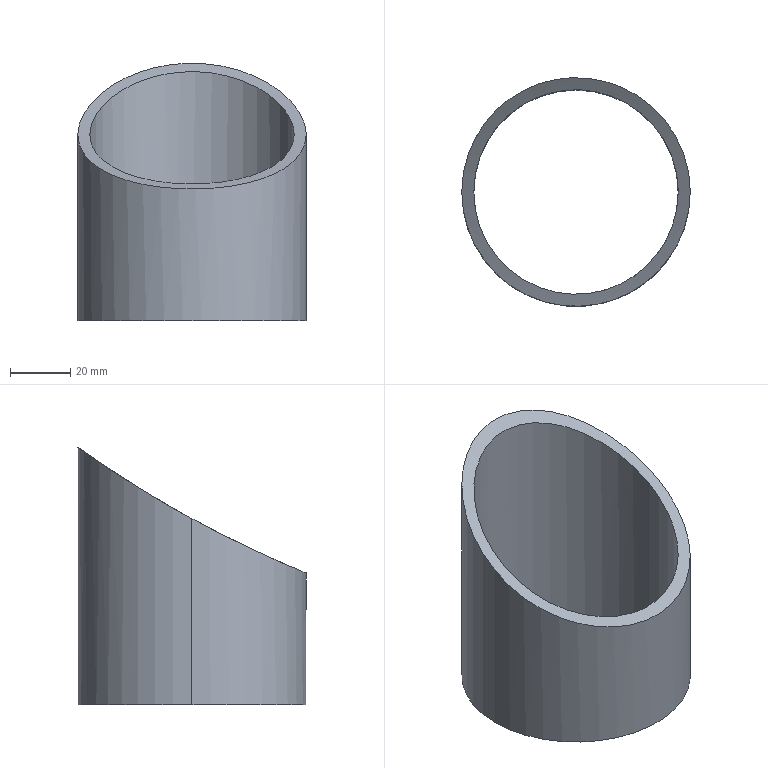Part | SolidWorks | features Extrusion 1, ICE 1 | 1 solid | 6 faces | box 76 x 76 x 85.679 mm | volume 57171 mm3 | cylinder 5 | plane 1 | commonest cylinder face diameters 68 x2 76 x2 759 x1
STEP:
#1=CARTESIAN_POINT('',(34.,0.,61.916));
#2=VERTEX_POINT('',#1);
#3=CARTESIAN_POINT('',(-34.,0.,61.916));
#4=VERTEX_POINT('',#3);
#5=CARTESIAN_POINT('',(34.,0.,61.916));
#6=CARTESIAN_POINT('',(34.,-2.054,60.794));
#7=CARTESIAN_POINT('',(33.815,-4.109,59.697));
#8=CARTESIAN_POINT('',(33.342,-6.678,58.355));
#9=CARTESIAN_POINT('',(33.235,-7.192,58.088));
#10=CARTESIAN_POINT('',(32.996,-8.22,57.557));
#11=CARTESIAN_POINT('',(32.863,-8.735,57.292));
#12=CARTESIAN_POINT('',(32.43,-10.268,56.509));
#13=CARTESIAN_POINT('',(32.094,-11.273,56.002));
#14=CARTESIAN_POINT('',(30.946,-14.241,54.519));
#15=CARTESIAN_POINT('',(29.995,-16.156,53.584));
#16=CARTESIAN_POINT('',(28.27,-18.92,52.261));
#17=CARTESIAN_POINT('',(27.645,-19.825,51.832));
#18=CARTESIAN_POINT('',(26.289,-21.59,51.004));
#19=CARTESIAN_POINT('',(25.57,-22.437,50.611));
#20=CARTESIAN_POINT('',(23.292,-24.868,49.493));
#21=CARTESIAN_POINT('',(21.611,-26.347,48.826));
#22=CARTESIAN_POINT('',(19.295,-28.,48.091));
#23=CARTESIAN_POINT('',(18.821,-28.321,47.949));
#24=CARTESIAN_POINT('',(17.851,-28.943,47.674));
#25=CARTESIAN_POINT('',(17.354,-29.244,47.542));
#26=CARTESIAN_POINT('',(15.847,-30.103,47.165));
#27=CARTESIAN_POINT('',(14.817,-30.623,46.939));
#28=CARTESIAN_POINT('',(11.652,-32.024,46.333));
#29=CARTESIAN_POINT('',(9.443,-32.748,46.024));
#30=CARTESIAN_POINT('',(6.549,-33.369,45.759));
#31=CARTESIAN_POINT('',(5.966,-33.478,45.713));
#32=CARTESIAN_POINT('',(4.802,-33.664,45.634));
#33=CARTESIAN_POINT('',(4.22,-33.742,45.601));
#34=CARTESIAN_POINT('',(2.469,-33.931,45.521));
#35=CARTESIAN_POINT('',(1.299,-33.995,45.494));
#36=CARTESIAN_POINT('',(-1.048,-34.004,45.49));
#37=CARTESIAN_POINT('',(-2.225,-33.948,45.514));
#38=CARTESIAN_POINT('',(-3.995,-33.77,45.589));
#39=CARTESIAN_POINT('',(-4.585,-33.695,45.621));
#40=CARTESIAN_POINT('',(-5.753,-33.515,45.697));
#41=CARTESIAN_POINT('',(-6.331,-33.41,45.742));
#42=CARTESIAN_POINT('',(-9.201,-32.815,45.995));
#43=CARTESIAN_POINT('',(-11.422,-32.11,46.296));
#44=CARTESIAN_POINT('',(-14.103,-30.943,46.801));
#45=CARTESIAN_POINT('',(-14.634,-30.695,46.908));
#46=CARTESIAN_POINT('',(-15.674,-30.177,47.134));
#47=CARTESIAN_POINT('',(-16.184,-29.906,47.252));
#48=CARTESIAN_POINT('',(-17.689,-29.059,47.623));
#49=CARTESIAN_POINT('',(-18.655,-28.448,47.892));
#50=CARTESIAN_POINT('',(-20.516,-27.136,48.475));
#51=CARTESIAN_POINT('',(-21.411,-26.436,48.788));
#52=CARTESIAN_POINT('',(-22.701,-25.318,49.293));
#53=CARTESIAN_POINT('',(-23.121,-24.934,49.467));
#54=CARTESIAN_POINT('',(-23.936,-24.153,49.823));
#55=CARTESIAN_POINT('',(-24.332,-23.755,50.005));
#56=CARTESIAN_POINT('',(-26.249,-21.725,50.938));
#57=CARTESIAN_POINT('',(-27.597,-19.981,51.754));
#58=CARTESIAN_POINT('',(-29.058,-17.661,52.863));
#59=CARTESIAN_POINT('',(-29.34,-17.189,53.09));
#60=CARTESIAN_POINT('',(-29.877,-16.237,53.55));
#61=CARTESIAN_POINT('',(-30.133,-15.758,53.783));
#62=CARTESIAN_POINT('',(-30.861,-14.309,54.491));
#63=CARTESIAN_POINT('',(-31.296,-13.33,54.975));
#64=CARTESIAN_POINT('',(-32.069,-11.346,55.965));
#65=CARTESIAN_POINT('',(-32.406,-10.341,56.472));
#66=CARTESIAN_POINT('',(-32.841,-8.816,57.251));
#67=CARTESIAN_POINT('',(-32.974,-8.304,57.513));
#68=CARTESIAN_POINT('',(-33.217,-7.275,58.045));
#69=CARTESIAN_POINT('',(-33.326,-6.757,58.314));
#70=CARTESIAN_POINT('',(-33.616,-5.201,59.126));
#71=CARTESIAN_POINT('',(-33.76,-4.163,59.674));
#72=CARTESIAN_POINT('',(-33.904,-2.603,60.507));
#73=CARTESIAN_POINT('',(-33.94,-2.083,60.786));
#74=CARTESIAN_POINT('',(-33.988,-1.042,61.348));
#75=CARTESIAN_POINT('',(-34.,-0.5196,61.632));
#76=CARTESIAN_POINT('',(-34.,0.,61.916));
#77=B_SPLINE_CURVE_WITH_KNOTS('',3,(#5,#6,#7,#8,#9,#10,#11,#12,#13,#14,#15,#16,#17,#18,#19,#20,#21,#22,#23,#24,#25,#26,#27,#28,#29,#30,#31,#32,#33,#34,#35,#36,#37,#38,#39,#40,#41,#42,#43,#44,#45,#46,#47,#48,#49,#50,#51,#52,#53,#54,#55,#56,#57,#58,#59,#60,#61,#62,#63,#64,#65,#66,#67,#68,#69,#70,#71,#72,#73,#74,#75,#76),.UNSPECIFIED.,.F.,.F.,(4,2,2,2,2,2,2,2,2,2,2,2,2,2,2,2,2,2,2,2,2,2,2,2,2,2,2,2,2,2,2,2,2,2,2,4),(0.1147,0.1217,0.1234,0.1252,0.1287,0.1356,0.1391,0.1426,0.1496,0.1513,0.153,0.1565,0.1635,0.1652,0.167,0.1705,0.1739,0.1757,0.1774,0.1844,0.1861,0.1879,0.1914,0.1948,0.1966,0.1983,0.2053,0.207,0.2088,0.2123,0.2157,0.2175,0.2192,0.2227,0.2245,0.2262),.UNSPECIFIED.);
#78=EDGE_CURVE('',#2,#4,#77,.T.);
#79=ORIENTED_EDGE('',*,*,#78,.F.);
#80=CARTESIAN_POINT('',(34.,0.,0.));
#81=VERTEX_POINT('',#80);
#82=CARTESIAN_POINT('',(34.,0.,500.));
#83=DIRECTION('',(0.,0.,-1.));
#84=VECTOR('',#83,1000.);
#85=LINE('',#82,#84);
#86=EDGE_CURVE('',#2,#81,#85,.T.);
#87=ORIENTED_EDGE('',*,*,#86,.T.);
#88=CARTESIAN_POINT('',(-34.,0.,0.));
#89=VERTEX_POINT('',#88);
#90=CARTESIAN_POINT('',(0.,0.,0.));
#91=DIRECTION('',(0.,0.,1.));
#92=DIRECTION('',(1.,0.,0.));
#93=AXIS2_PLACEMENT_3D('',#90,#91,#92);
#94=CIRCLE('',#93,34.);
#95=EDGE_CURVE('',#89,#81,#94,.T.);
#96=ORIENTED_EDGE('',*,*,#95,.F.);
#97=CARTESIAN_POINT('',(-34.,0.,500.));
#98=DIRECTION('',(0.,0.,-1.));
#99=VECTOR('',#98,1000.);
#100=LINE('',#97,#99);
#101=EDGE_CURVE('',#4,#89,#100,.T.);
#102=ORIENTED_EDGE('',*,*,#101,.F.);
#103=EDGE_LOOP('',(#79,#87,#96,#102));
#104=FACE_OUTER_BOUND('',#103,.T.);
#105=CARTESIAN_POINT('',(0.,0.,500.));
#106=DIRECTION('',(0.,0.,-1.));
#107=DIRECTION('',(-1.,0.,0.));
#108=AXIS2_PLACEMENT_3D('',#105,#106,#107);
#109=CYLINDRICAL_SURFACE('',#108,34.);
#110=ADVANCED_FACE('',(#104),#109,.F.);
#111=CARTESIAN_POINT('',(-38.,0.,61.916));
#112=VERTEX_POINT('',#111);
#113=CARTESIAN_POINT('',(38.,0.,61.916));
#114=VERTEX_POINT('',#113);
#115=CARTESIAN_POINT('',(-38.,0.,61.916));
#116=CARTESIAN_POINT('',(-38.,2.395,63.223));
#117=CARTESIAN_POINT('',(-37.776,4.737,64.535));
#118=CARTESIAN_POINT('',(-36.913,9.322,67.167));
#119=CARTESIAN_POINT('',(-36.274,11.565,68.486));
#120=CARTESIAN_POINT('',(-35.208,14.308,70.136));
#121=CARTESIAN_POINT('',(-34.982,14.853,70.466));
#122=CARTESIAN_POINT('',(-34.501,15.938,71.126));
#123=CARTESIAN_POINT('',(-34.246,16.478,71.457));
#124=CARTESIAN_POINT('',(-33.446,18.078,72.441));
#125=CARTESIAN_POINT('',(-32.864,19.115,73.086));
#126=CARTESIAN_POINT('',(-30.976,22.14,74.988));
#127=CARTESIAN_POINT('',(-29.527,24.043,76.211));
#128=CARTESIAN_POINT('',(-27.047,26.719,77.961));
#129=CARTESIAN_POINT('',(-26.168,27.582,78.53));
#130=CARTESIAN_POINT('',(-24.3,29.242,79.635));
#131=CARTESIAN_POINT('',(-23.325,30.026,80.162));
#132=CARTESIAN_POINT('',(-20.274,32.238,81.658));
#133=CARTESIAN_POINT('',(-18.075,33.529,82.546));
#134=CARTESIAN_POINT('',(-15.085,34.884,83.487));
#135=CARTESIAN_POINT('',(-14.476,35.141,83.666));
#136=CARTESIAN_POINT('',(-13.25,35.621,84.002));
#137=CARTESIAN_POINT('',(-12.631,35.845,84.159));
#138=CARTESIAN_POINT('',(-10.757,36.469,84.596));
#139=CARTESIAN_POINT('',(-9.484,36.822,84.845));
#140=CARTESIAN_POINT('',(-6.887,37.394,85.249));
#141=CARTESIAN_POINT('',(-5.565,37.615,85.406));
#142=CARTESIAN_POINT('',(-3.541,37.841,85.566));
#143=CARTESIAN_POINT('',(-2.858,37.899,85.607));
#144=CARTESIAN_POINT('',(-1.496,37.977,85.662));
#145=CARTESIAN_POINT('',(-0.8168,37.997,85.677));
#146=CARTESIAN_POINT('',(2.569,38.01,85.686));
#147=CARTESIAN_POINT('',(5.25,37.733,85.489));
#148=CARTESIAN_POINT('',(9.227,36.888,84.891));
#149=CARTESIAN_POINT('',(10.52,36.539,84.645));
#150=CARTESIAN_POINT('',(13.037,35.718,84.069));
#151=CARTESIAN_POINT('',(14.263,35.246,83.739));
#152=CARTESIAN_POINT('',(16.054,34.448,83.185));
#153=CARTESIAN_POINT('',(16.643,34.168,82.99));
#154=CARTESIAN_POINT('',(17.806,33.576,82.582));
#155=CARTESIAN_POINT('',(18.378,33.266,82.368));
#156=CARTESIAN_POINT('',(20.054,32.303,81.707));
#157=CARTESIAN_POINT('',(21.122,31.614,81.236));
#158=CARTESIAN_POINT('',(23.17,30.145,80.242));
#159=CARTESIAN_POINT('',(24.149,29.366,79.719));
#160=CARTESIAN_POINT('',(26.021,27.721,78.623));
#161=CARTESIAN_POINT('',(26.915,26.853,78.049));
#162=CARTESIAN_POINT('',(29.427,24.167,76.291));
#163=CARTESIAN_POINT('',(30.894,22.255,75.061));
#164=CARTESIAN_POINT('',(32.489,19.719,73.466));
#165=CARTESIAN_POINT('',(32.795,19.205,73.144));
#166=CARTESIAN_POINT('',(33.385,18.161,72.494));
#167=CARTESIAN_POINT('',(33.667,17.631,72.166));
#168=CARTESIAN_POINT('',(34.473,16.033,71.182));
#169=CARTESIAN_POINT('',(34.955,14.951,70.523));
#170=CARTESIAN_POINT('',(36.244,11.658,68.541));
#171=CARTESIAN_POINT('',(36.895,9.399,67.211));
#172=CARTESIAN_POINT('',(37.556,5.911,65.209));
#173=CARTESIAN_POINT('',(37.723,4.728,64.538));
#174=CARTESIAN_POINT('',(37.945,2.365,63.215));
#175=CARTESIAN_POINT('',(38.,1.183,62.562));
#176=CARTESIAN_POINT('',(38.,0.,61.916));
#177=B_SPLINE_CURVE_WITH_KNOTS('',3,(#115,#116,#117,#118,#119,#120,#121,#122,#123,#124,#125,#126,#127,#128,#129,#130,#131,#132,#133,#134,#135,#136,#137,#138,#139,#140,#141,#142,#143,#144,#145,#146,#147,#148,#149,#150,#151,#152,#153,#154,#155,#156,#157,#158,#159,#160,#161,#162,#163,#164,#165,#166,#167,#168,#169,#170,#171,#172,#173,#174,#175,#176),.UNSPECIFIED.,.F.,.F.,(4,2,2,2,2,2,2,2,2,2,2,2,2,2,2,2,2,2,2,2,2,2,2,2,2,2,2,2,2,2,4),(0.,0.00803,0.01606,0.01807,0.02008,0.02409,0.03212,0.03614,0.04015,0.04818,0.05019,0.0522,0.05621,0.06023,0.06223,0.06424,0.07227,0.07629,0.0803,0.08231,0.08432,0.08833,0.09235,0.09636,0.1044,0.1064,0.1084,0.1124,0.1205,0.1245,0.1285),.UNSPECIFIED.);
#178=EDGE_CURVE('',#112,#114,#177,.T.);
#179=ORIENTED_EDGE('',*,*,#178,.T.);
#180=CARTESIAN_POINT('',(38.,0.,0.));
#181=VERTEX_POINT('',#180);
#182=CARTESIAN_POINT('',(38.,0.,500.));
#183=DIRECTION('',(0.,0.,-1.));
#184=VECTOR('',#183,1000.);
#185=LINE('',#182,#184);
#186=EDGE_CURVE('',#114,#181,#185,.T.);
#187=ORIENTED_EDGE('',*,*,#186,.T.);
#188=CARTESIAN_POINT('',(-38.,0.,0.));
#189=VERTEX_POINT('',#188);
#190=CARTESIAN_POINT('',(0.,0.,0.));
#191=DIRECTION('',(0.,0.,1.));
#192=DIRECTION('',(1.,0.,0.));
#193=AXIS2_PLACEMENT_3D('',#190,#191,#192);
#194=CIRCLE('',#193,38.);
#195=EDGE_CURVE('',#181,#189,#194,.T.);
#196=ORIENTED_EDGE('',*,*,#195,.T.);
#197=CARTESIAN_POINT('',(-38.,0.,500.));
#198=DIRECTION('',(0.,0.,-1.));
#199=VECTOR('',#198,1000.);
#200=LINE('',#197,#199);
#201=EDGE_CURVE('',#112,#189,#200,.T.);
#202=ORIENTED_EDGE('',*,*,#201,.F.);
#203=EDGE_LOOP('',(#179,#187,#196,#202));
#204=FACE_OUTER_BOUND('',#203,.T.);
#205=CARTESIAN_POINT('',(0.,0.,500.));
#206=DIRECTION('',(0.,0.,-1.));
#207=DIRECTION('',(-1.,0.,0.));
#208=AXIS2_PLACEMENT_3D('',#205,#206,#207);
#209=CYLINDRICAL_SURFACE('',#208,38.);
#210=ADVANCED_FACE('',(#204),#209,.T.);
#211=CARTESIAN_POINT('',(0.,0.,0.));
#212=DIRECTION('',(0.,0.,1.));
#213=DIRECTION('',(1.,0.,0.));
#214=AXIS2_PLACEMENT_3D('',#211,#212,#213);
#215=CIRCLE('',#214,38.);
#216=EDGE_CURVE('',#189,#181,#215,.T.);
#217=ORIENTED_EDGE('',*,*,#216,.F.);
#218=ORIENTED_EDGE('',*,*,#195,.F.);
#219=EDGE_LOOP('',(#217,#218));
#220=FACE_OUTER_BOUND('',#219,.T.);
#221=ORIENTED_EDGE('',*,*,#95,.T.);
#222=CARTESIAN_POINT('',(0.,0.,0.));
#223=DIRECTION('',(0.,0.,1.));
#224=DIRECTION('',(1.,0.,0.));
#225=AXIS2_PLACEMENT_3D('',#222,#223,#224);
#226=CIRCLE('',#225,34.);
#227=EDGE_CURVE('',#81,#89,#226,.T.);
#228=ORIENTED_EDGE('',*,*,#227,.T.);
#229=EDGE_LOOP('',(#221,#228));
#230=FACE_BOUND('',#229,.T.);
#231=CARTESIAN_POINT('',(0.,0.,0.));
#232=DIRECTION('',(0.,0.,1.));
#233=DIRECTION('',(1.,0.,0.));
#234=AXIS2_PLACEMENT_3D('',#231,#232,#233);
#235=PLANE('',#234);
#236=ADVANCED_FACE('',(#220,#230),#235,.F.);
#237=ORIENTED_EDGE('',*,*,#186,.F.);
#238=CARTESIAN_POINT('',(38.,0.,61.916));
#239=CARTESIAN_POINT('',(38.,-2.292,60.664));
#240=CARTESIAN_POINT('',(37.794,-4.587,59.442));
#241=CARTESIAN_POINT('',(37.265,-7.459,57.949));
#242=CARTESIAN_POINT('',(37.146,-8.034,57.653));
#243=CARTESIAN_POINT('',(36.878,-9.184,57.063));
#244=CARTESIAN_POINT('',(36.73,-9.76,56.769));
#245=CARTESIAN_POINT('',(36.246,-11.472,55.901));
#246=CARTESIAN_POINT('',(35.871,-12.596,55.339));
#247=CARTESIAN_POINT('',(34.589,-15.914,53.699));
#248=CARTESIAN_POINT('',(33.525,-18.055,52.667));
#249=CARTESIAN_POINT('',(31.916,-20.633,51.453));
#250=CARTESIAN_POINT('',(31.58,-21.144,51.213));
#251=CARTESIAN_POINT('',(30.879,-22.155,50.743));
#252=CARTESIAN_POINT('',(30.514,-22.656,50.51));
#253=CARTESIAN_POINT('',(29.377,-24.136,49.829));
#254=CARTESIAN_POINT('',(28.573,-25.083,49.398));
#255=CARTESIAN_POINT('',(26.024,-27.802,48.174));
#256=CARTESIAN_POINT('',(24.144,-29.455,47.446));
#257=CARTESIAN_POINT('',(21.552,-31.304,46.644));
#258=CARTESIAN_POINT('',(21.021,-31.663,46.49));
#259=CARTESIAN_POINT('',(19.935,-32.358,46.191));
#260=CARTESIAN_POINT('',(19.379,-32.693,46.047));
#261=CARTESIAN_POINT('',(17.696,-33.653,45.638));
#262=CARTESIAN_POINT('',(16.546,-34.233,45.393));
#263=CARTESIAN_POINT('',(13.01,-35.796,44.735));
#264=CARTESIAN_POINT('',(10.541,-36.605,44.401));
#265=CARTESIAN_POINT('',(5.364,-37.713,43.944));
#266=CARTESIAN_POINT('',(2.759,-37.99,43.83));
#267=CARTESIAN_POINT('',(-1.172,-38.005,43.824));
#268=CARTESIAN_POINT('',(-2.486,-37.942,43.85));
#269=CARTESIAN_POINT('',(-4.464,-37.743,43.932));
#270=CARTESIAN_POINT('',(-5.122,-37.659,43.966));
#271=CARTESIAN_POINT('',(-6.424,-37.459,44.048));
#272=CARTESIAN_POINT('',(-7.07,-37.342,44.096));
#273=CARTESIAN_POINT('',(-10.273,-36.679,44.37));
#274=CARTESIAN_POINT('',(-12.753,-35.891,44.696));
#275=CARTESIAN_POINT('',(-15.751,-34.588,45.243));
#276=CARTESIAN_POINT('',(-16.344,-34.312,45.36));
#277=CARTESIAN_POINT('',(-17.506,-33.734,45.604));
#278=CARTESIAN_POINT('',(-18.076,-33.432,45.732));
#279=CARTESIAN_POINT('',(-19.757,-32.486,46.135));
#280=CARTESIAN_POINT('',(-20.837,-31.803,46.428));
#281=CARTESIAN_POINT('',(-22.919,-30.337,47.063));
#282=CARTESIAN_POINT('',(-23.92,-29.554,47.405));
#283=CARTESIAN_POINT('',(-25.363,-28.304,47.956));
#284=CARTESIAN_POINT('',(-25.833,-27.876,48.146));
#285=CARTESIAN_POINT('',(-26.745,-27.002,48.535));
#286=CARTESIAN_POINT('',(-27.187,-26.557,48.735));
#287=CARTESIAN_POINT('',(-29.332,-24.287,49.756));
#288=CARTESIAN_POINT('',(-30.84,-22.337,50.651));
#289=CARTESIAN_POINT('',(-32.476,-19.741,51.873));
#290=CARTESIAN_POINT('',(-32.791,-19.213,52.123));
#291=CARTESIAN_POINT('',(-33.392,-18.148,52.63));
#292=CARTESIAN_POINT('',(-33.678,-17.612,52.887));
#293=CARTESIAN_POINT('',(-34.492,-15.992,53.668));
#294=CARTESIAN_POINT('',(-34.979,-14.897,54.202));
#295=CARTESIAN_POINT('',(-35.843,-12.678,55.298));
#296=CARTESIAN_POINT('',(-36.22,-11.554,55.86));
#297=CARTESIAN_POINT('',(-36.706,-9.848,56.724));
#298=CARTESIAN_POINT('',(-36.855,-9.276,57.015));
#299=CARTESIAN_POINT('',(-37.126,-8.126,57.605));
#300=CARTESIAN_POINT('',(-37.248,-7.546,57.904));
#301=CARTESIAN_POINT('',(-37.572,-5.808,58.807));
#302=CARTESIAN_POINT('',(-37.733,-4.648,59.417));
#303=CARTESIAN_POINT('',(-37.893,-2.906,60.345));
#304=CARTESIAN_POINT('',(-37.933,-2.325,60.656));
#305=CARTESIAN_POINT('',(-37.987,-1.163,61.283));
#306=CARTESIAN_POINT('',(-38.,-0.58,61.599));
#307=CARTESIAN_POINT('',(-38.,0.,61.916));
#308=B_SPLINE_CURVE_WITH_KNOTS('',3,(#238,#239,#240,#241,#242,#243,#244,#245,#246,#247,#248,#249,#250,#251,#252,#253,#254,#255,#256,#257,#258,#259,#260,#261,#262,#263,#264,#265,#266,#267,#268,#269,#270,#271,#272,#273,#274,#275,#276,#277,#278,#279,#280,#281,#282,#283,#284,#285,#286,#287,#288,#289,#290,#291,#292,#293,#294,#295,#296,#297,#298,#299,#300,#301,#302,#303,#304,#305,#306,#307),.UNSPECIFIED.,.F.,.F.,(4,2,2,2,2,2,2,2,2,2,2,2,2,2,2,2,2,2,2,2,2,2,2,2,2,2,2,2,2,2,2,2,2,2,4),(0.1285,0.1363,0.1382,0.1401,0.144,0.1518,0.1538,0.1557,0.1596,0.1674,0.1693,0.1713,0.1751,0.1829,0.1907,0.1946,0.1965,0.1985,0.2063,0.2082,0.2101,0.214,0.2179,0.2199,0.2218,0.2296,0.2315,0.2335,0.2374,0.2413,0.2432,0.2451,0.249,0.251,0.2529),.UNSPECIFIED.);
#309=EDGE_CURVE('',#114,#112,#308,.T.);
#310=ORIENTED_EDGE('',*,*,#309,.T.);
#311=ORIENTED_EDGE('',*,*,#201,.T.);
#312=ORIENTED_EDGE('',*,*,#216,.T.);
#313=EDGE_LOOP('',(#237,#310,#311,#312));
#314=FACE_OUTER_BOUND('',#313,.T.);
#315=CARTESIAN_POINT('',(0.,0.,500.));
#316=DIRECTION('',(0.,0.,-1.));
#317=DIRECTION('',(-1.,0.,0.));
#318=AXIS2_PLACEMENT_3D('',#315,#316,#317);
#319=CYLINDRICAL_SURFACE('',#318,38.);
#320=ADVANCED_FACE('',(#314),#319,.T.);
#321=ORIENTED_EDGE('',*,*,#86,.F.);
#322=CARTESIAN_POINT('',(-34.,0.,61.916));
#323=CARTESIAN_POINT('',(-34.,2.139,63.083));
#324=CARTESIAN_POINT('',(-33.8,4.231,64.253));
#325=CARTESIAN_POINT('',(-33.03,8.33,66.593));
#326=CARTESIAN_POINT('',(-32.459,10.337,67.764));
#327=CARTESIAN_POINT('',(-31.506,12.792,69.226));
#328=CARTESIAN_POINT('',(-31.303,13.281,69.518));
#329=CARTESIAN_POINT('',(-30.873,14.252,70.102));
#330=CARTESIAN_POINT('',(-30.645,14.736,70.395));
#331=CARTESIAN_POINT('',(-29.929,16.169,71.265));
#332=CARTESIAN_POINT('',(-29.408,17.098,71.836));
#333=CARTESIAN_POINT('',(-27.716,19.808,73.515));
#334=CARTESIAN_POINT('',(-26.419,21.513,74.592));
#335=CARTESIAN_POINT('',(-24.196,23.911,76.131));
#336=CARTESIAN_POINT('',(-23.409,24.684,76.631));
#337=CARTESIAN_POINT('',(-21.734,26.17,77.601));
#338=CARTESIAN_POINT('',(-20.86,26.872,78.062));
#339=CARTESIAN_POINT('',(-18.127,28.853,79.373));
#340=CARTESIAN_POINT('',(-16.157,30.008,80.149));
#341=CARTESIAN_POINT('',(-13.482,31.218,80.969));
#342=CARTESIAN_POINT('',(-12.937,31.448,81.125));
#343=CARTESIAN_POINT('',(-11.84,31.877,81.417));
#344=CARTESIAN_POINT('',(-11.286,32.078,81.553));
#345=CARTESIAN_POINT('',(-9.609,32.635,81.934));
#346=CARTESIAN_POINT('',(-8.471,32.949,82.15));
#347=CARTESIAN_POINT('',(-6.15,33.46,82.502));
#348=CARTESIAN_POINT('',(-4.969,33.657,82.637));
#349=CARTESIAN_POINT('',(-3.161,33.858,82.776));
#350=CARTESIAN_POINT('',(-2.551,33.91,82.812));
#351=CARTESIAN_POINT('',(-1.335,33.979,82.86));
#352=CARTESIAN_POINT('',(-0.7283,33.998,82.873));
#353=CARTESIAN_POINT('',(2.296,34.009,82.88));
#354=CARTESIAN_POINT('',(4.69,33.762,82.709));
#355=CARTESIAN_POINT('',(8.242,33.008,82.191));
#356=CARTESIAN_POINT('',(9.399,32.697,81.977));
#357=CARTESIAN_POINT('',(11.649,31.964,81.476));
#358=CARTESIAN_POINT('',(12.746,31.542,81.188));
#359=CARTESIAN_POINT('',(14.348,30.83,80.705));
#360=CARTESIAN_POINT('',(14.875,30.579,80.536));
#361=CARTESIAN_POINT('',(15.915,30.051,80.18));
#362=CARTESIAN_POINT('',(16.428,29.774,79.993));
#363=CARTESIAN_POINT('',(17.929,28.912,79.415));
#364=CARTESIAN_POINT('',(18.886,28.295,79.004));
#365=CARTESIAN_POINT('',(20.72,26.98,78.133));
#366=CARTESIAN_POINT('',(21.597,26.283,77.675));
#367=CARTESIAN_POINT('',(23.274,24.811,76.714));
#368=CARTESIAN_POINT('',(24.075,24.033,76.21));
#369=CARTESIAN_POINT('',(26.328,21.625,74.663));
#370=CARTESIAN_POINT('',(27.643,19.912,73.58));
#371=CARTESIAN_POINT('',(29.07,17.641,72.172));
#372=CARTESIAN_POINT('',(29.345,17.181,71.888));
#373=CARTESIAN_POINT('',(29.872,16.247,71.315));
#374=CARTESIAN_POINT('',(30.125,15.772,71.025));
#375=CARTESIAN_POINT('',(30.847,14.339,70.153));
#376=CARTESIAN_POINT('',(31.279,13.37,69.57));
#377=CARTESIAN_POINT('',(32.432,10.421,67.813));
#378=CARTESIAN_POINT('',(33.014,8.4,66.633));
#379=CARTESIAN_POINT('',(33.604,5.283,64.853));
#380=CARTESIAN_POINT('',(33.753,4.226,64.256));
#381=CARTESIAN_POINT('',(33.951,2.113,63.076));
#382=CARTESIAN_POINT('',(34.,1.057,62.493));
#383=CARTESIAN_POINT('',(34.,0.,61.916));
#384=B_SPLINE_CURVE_WITH_KNOTS('',3,(#322,#323,#324,#325,#326,#327,#328,#329,#330,#331,#332,#333,#334,#335,#336,#337,#338,#339,#340,#341,#342,#343,#344,#345,#346,#347,#348,#349,#350,#351,#352,#353,#354,#355,#356,#357,#358,#359,#360,#361,#362,#363,#364,#365,#366,#367,#368,#369,#370,#371,#372,#373,#374,#375,#376,#377,#378,#379,#380,#381,#382,#383),.UNSPECIFIED.,.F.,.F.,(4,2,2,2,2,2,2,2,2,2,2,2,2,2,2,2,2,2,2,2,2,2,2,2,2,2,2,2,2,2,4),(0.,0.00717,0.01434,0.01613,0.01793,0.02151,0.02868,0.03227,0.03585,0.04302,0.04481,0.04661,0.05019,0.05378,0.05557,0.05736,0.06453,0.06812,0.0717,0.07349,0.07529,0.07887,0.08246,0.08604,0.09321,0.095,0.0968,0.1004,0.1076,0.1111,0.1147),.UNSPECIFIED.);
#385=EDGE_CURVE('',#4,#2,#384,.T.);
#386=ORIENTED_EDGE('',*,*,#385,.F.);
#387=ORIENTED_EDGE('',*,*,#101,.T.);
#388=ORIENTED_EDGE('',*,*,#227,.F.);
#389=EDGE_LOOP('',(#321,#386,#387,#388));
#390=FACE_OUTER_BOUND('',#389,.T.);
#391=CARTESIAN_POINT('',(0.,0.,500.));
#392=DIRECTION('',(0.,0.,-1.));
#393=DIRECTION('',(-1.,0.,0.));
#394=AXIS2_PLACEMENT_3D('',#391,#392,#393);
#395=CYLINDRICAL_SURFACE('',#394,34.);
#396=ADVANCED_FACE('',(#390),#395,.F.);
#397=ORIENTED_EDGE('',*,*,#385,.T.);
#398=ORIENTED_EDGE('',*,*,#78,.T.);
#399=EDGE_LOOP('',(#397,#398));
#400=FACE_BOUND('',#399,.T.);
#401=ORIENTED_EDGE('',*,*,#178,.F.);
#402=ORIENTED_EDGE('',*,*,#309,.F.);
#403=EDGE_LOOP('',(#401,#402));
#404=FACE_OUTER_BOUND('',#403,.T.);
#405=CARTESIAN_POINT('',(-50.,-181.865,395.));
#406=DIRECTION('',(1.,0.,0.));
#407=DIRECTION('',(0.,0.,-1.));
#408=AXIS2_PLACEMENT_3D('',#405,#406,#407);
#409=CYLINDRICAL_SURFACE('',#408,379.5);
#410=ADVANCED_FACE('',(#400,#404),#409,.F.);
#411=CLOSED_SHELL('',(#110,#210,#236,#320,#396,#410));
#412=MANIFOLD_SOLID_BREP('',#411);
#413=CARTESIAN_POINT('',(0.,0.,0.));
#414=DIRECTION('',(0.,0.,1.));
#415=DIRECTION('',(1.,0.,0.));
#416=AXIS2_PLACEMENT_3D('',#413,#414,#415);
#417=(LENGTH_UNIT()NAMED_UNIT(*)SI_UNIT(.MILLI.,.METRE.));
#418=UNCERTAINTY_MEASURE_WITH_UNIT(LENGTH_MEASURE(0.00001),#417,'','');
#419=(NAMED_UNIT(*)PLANE_ANGLE_UNIT()SI_UNIT($,.RADIAN.));
#420=(NAMED_UNIT(*)SI_UNIT($,.STERADIAN.)SOLID_ANGLE_UNIT());
#421=(GEOMETRIC_REPRESENTATION_CONTEXT(3)GLOBAL_UNCERTAINTY_ASSIGNED_CONTEXT((#418))GLOBAL_UNIT_ASSIGNED_CONTEXT((#417,#419,#420))REPRESENTATION_CONTEXT('',''));
#422=ADVANCED_BREP_SHAPE_REPRESENTATION('',(#412,#416),#421);